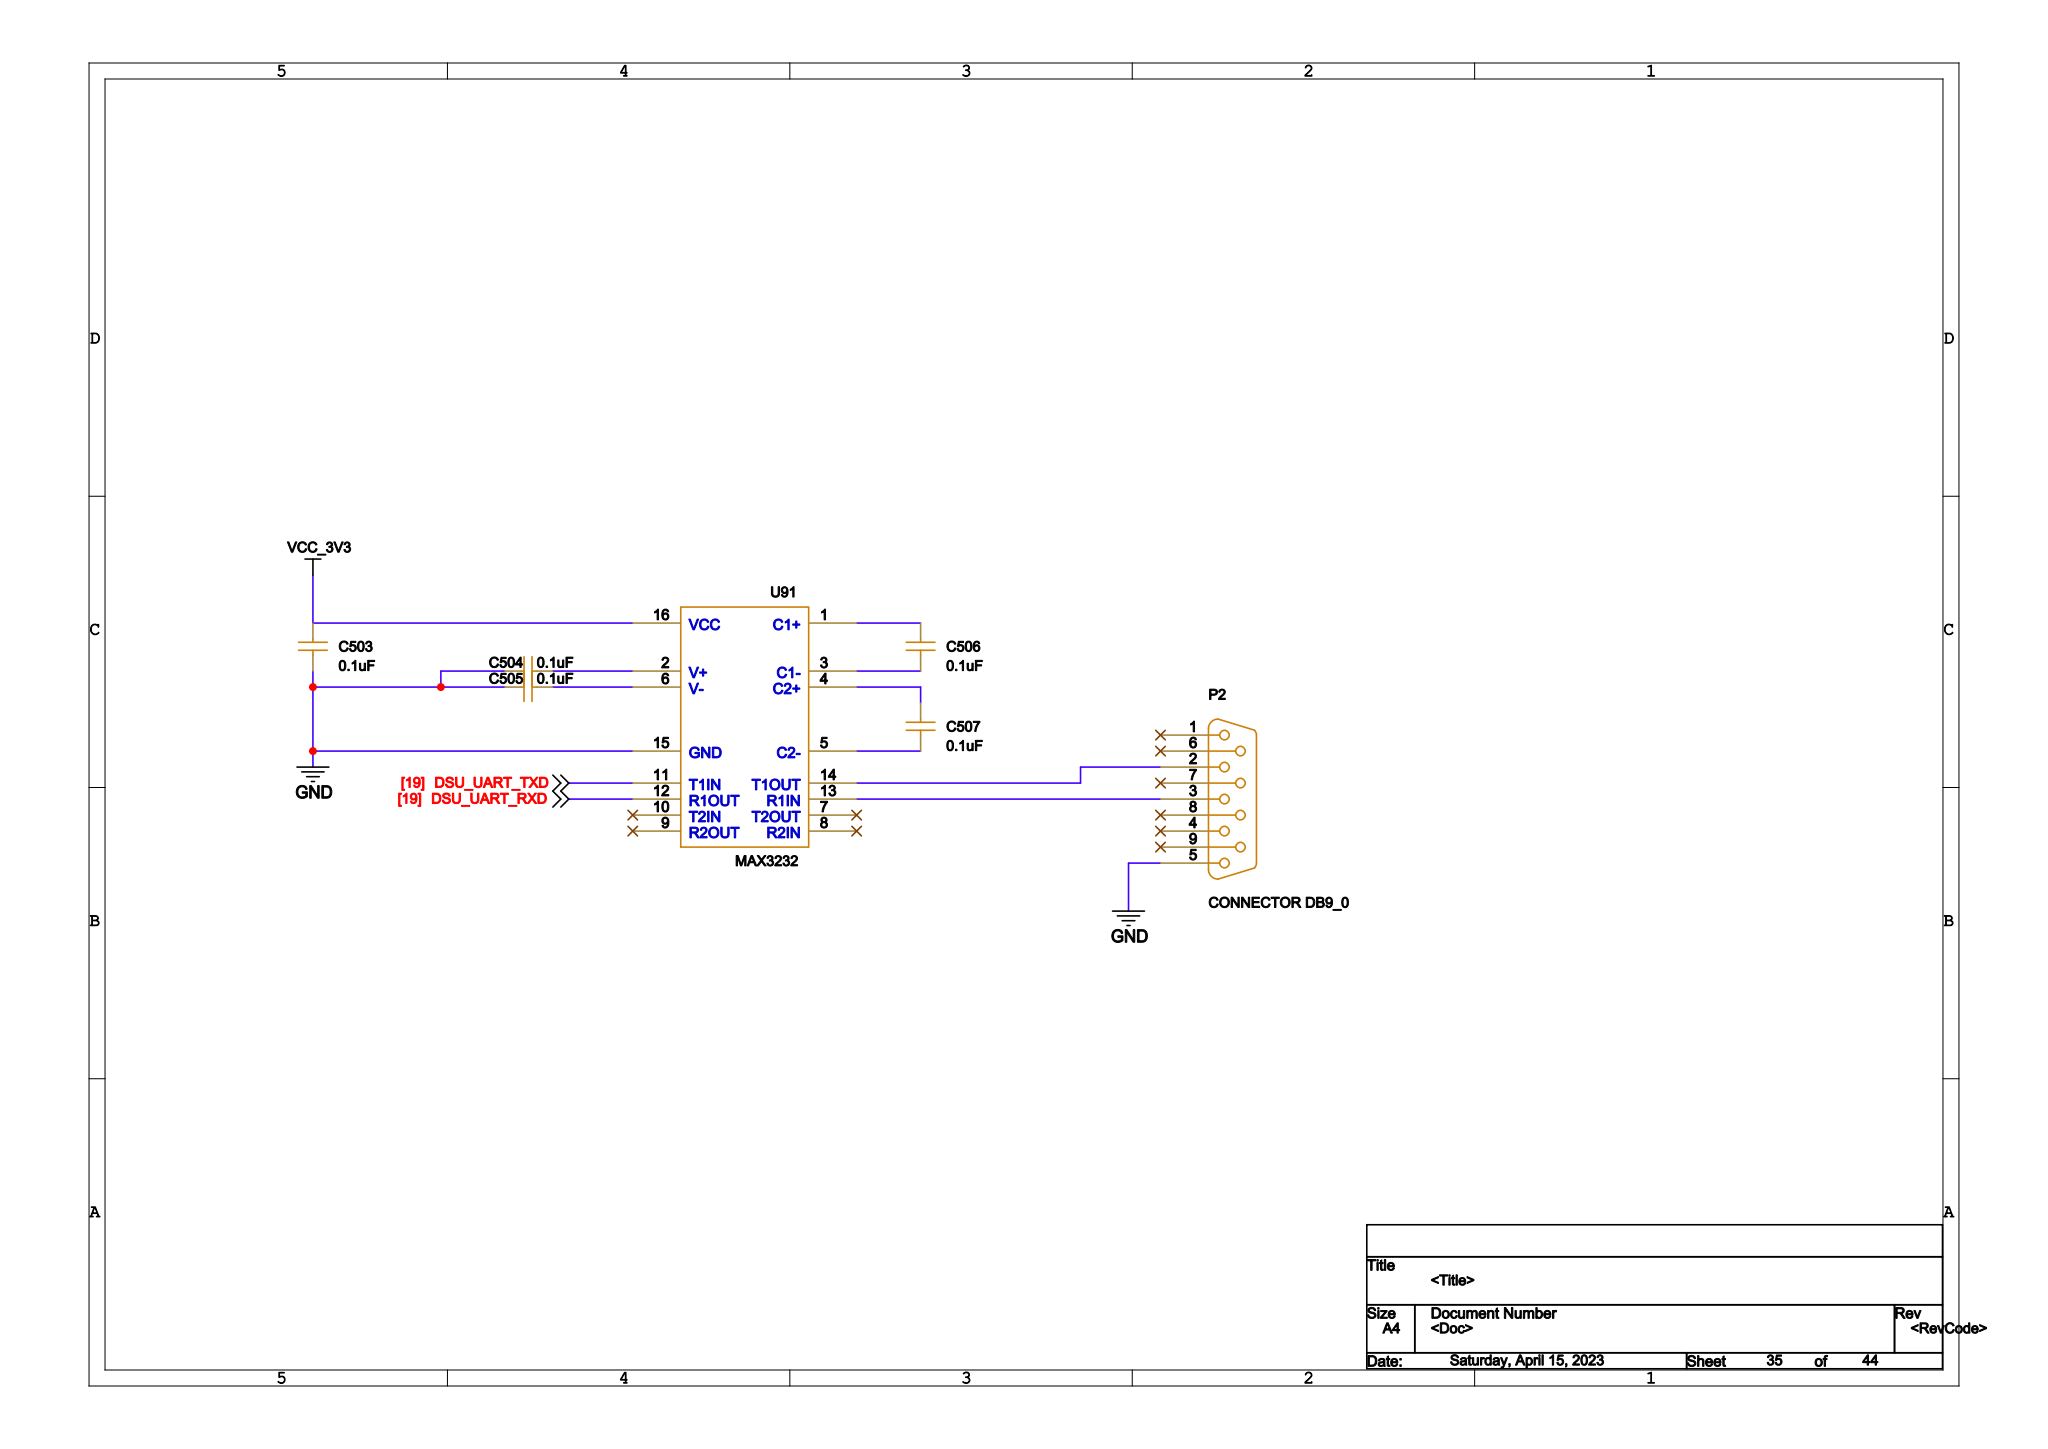Circuit board | Cadence Allegro | 1034 parts | 912 nets | one sheet of the schematic
Parts on this sheet (reference | value | footprint):
C503 | 0.1uF | C0402
C504 | 0.1uF | C0402
C505 | 0.1uF | C0402
C506 | 0.1uF | C0402
C507 | 0.1uF | C0402
U91 | MAX3232 | MAX3232
Nets of these parts (net: part-pin ...):
GND: C503-2 C504-1 C505-1 U91-15
VCC_3V3: C503-1 U91-16
N14265247: C504-2 U91-2
N14265267: C505-2 U91-6
N14265167: C506-1 U91-1
N14265251: C506-2 U91-3
N14265271: C507-1 U91-4
N14265303: C507-2 U91-5
N14265373: U91-13
N14265347: U91-14
DSU_UART_TXD: U91-11
DSU_UART_RXD: U91-12